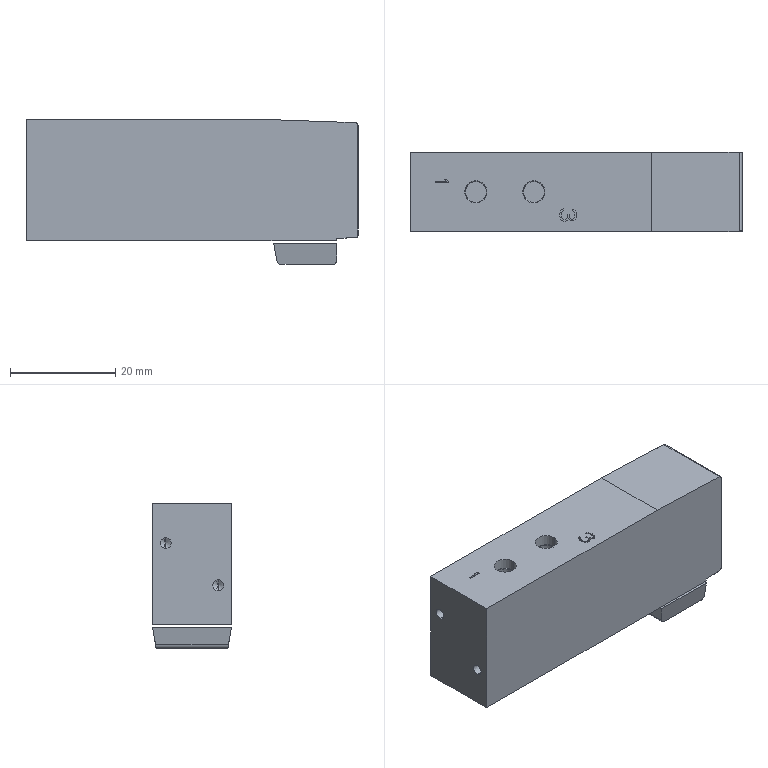Part | STEP file | COMPOUND | 2 solids | 152 faces | box 63 x 15 x 27.5 mm | volume 21811 mm3 | plane 116 | cylinder 24 | cone 8 | sphere 4 | commonest cylinder face diameters 1 x8 4 x6 2.05 x4 4.2 x4 1.6 x2